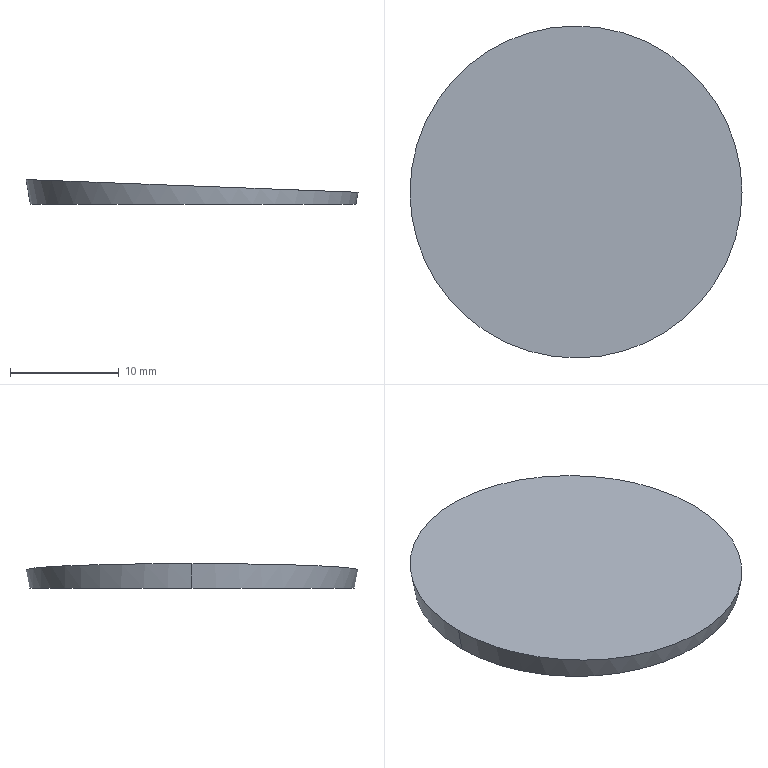Part | Creo | 1 solid | 4 faces | box 30.6 x 30.599 x 2.285 mm | volume 1225 mm3 | plane 2 | cone 2
STEP:
#1=CARTESIAN_POINT('',(15.,35.,35.405));
#2=VERTEX_POINT('',#1);
#3=CARTESIAN_POINT('',(-15.,35.,35.405));
#4=VERTEX_POINT('',#3);
#5=CARTESIAN_POINT('',(0.,35.,35.405));
#6=DIRECTION('',(0.,0.,-1.));
#7=DIRECTION('',(1.,0.,0.));
#8=AXIS2_PLACEMENT_3D('',#5,#6,#7);
#9=CIRCLE('',#8,15.);
#10=EDGE_CURVE('',#2,#4,#9,.T.);
#11=ORIENTED_EDGE('',*,*,#10,.F.);
#12=CARTESIAN_POINT('',(0.,35.,35.405));
#13=DIRECTION('',(0.,0.,-1.));
#14=DIRECTION('',(-1.,0.,0.));
#15=AXIS2_PLACEMENT_3D('',#12,#13,#14);
#16=CIRCLE('',#15,15.);
#17=EDGE_CURVE('',#4,#2,#16,.T.);
#18=ORIENTED_EDGE('',*,*,#17,.F.);
#19=EDGE_LOOP('',(#11,#18));
#20=FACE_OUTER_BOUND('',#19,.F.);
#21=CARTESIAN_POINT('',(0.,35.,35.405));
#22=DIRECTION('',(0.,0.,-1.));
#23=DIRECTION('',(-1.,0.,0.));
#24=AXIS2_PLACEMENT_3D('',#21,#22,#23);
#25=PLANE('',#24);
#26=ADVANCED_FACE('',(#20),#25,.T.);
#27=ORIENTED_EDGE('',*,*,#10,.T.);
#28=CARTESIAN_POINT('',(-15.403,35.,37.69));
#29=VERTEX_POINT('',#28);
#30=CARTESIAN_POINT('',(-15.,35.,35.405));
#31=DIRECTION('',(-0.1736,0.,0.9848));
#32=VECTOR('',#31,2.32);
#33=LINE('',#30,#32);
#34=EDGE_CURVE('',#4,#29,#33,.T.);
#35=ORIENTED_EDGE('',*,*,#34,.T.);
#36=CARTESIAN_POINT('',(15.197,35.,36.522));
#37=VERTEX_POINT('',#36);
#38=CARTESIAN_POINT('',(-15.403,35.,37.69));
#39=CARTESIAN_POINT('',(-15.403,34.098,37.69));
#40=CARTESIAN_POINT('',(-15.243,32.228,37.684));
#41=CARTESIAN_POINT('',(-14.431,29.351,37.653));
#42=CARTESIAN_POINT('',(-13.006,26.578,37.599));
#43=CARTESIAN_POINT('',(-11.,24.103,37.522));
#44=CARTESIAN_POINT('',(-8.525,22.097,37.428));
#45=CARTESIAN_POINT('',(-6.214,20.91,37.34));
#46=CARTESIAN_POINT('',(-4.314,20.266,37.267));
#47=CARTESIAN_POINT('',(-2.884,19.932,37.212));
#48=CARTESIAN_POINT('',(-1.708,19.772,37.168));
#49=CARTESIAN_POINT('',(-0.7827,19.71,37.132));
#50=CARTESIAN_POINT('',(-0.103,19.695,37.106));
#51=CARTESIAN_POINT('',(0.5768,19.71,37.08));
#52=CARTESIAN_POINT('',(1.502,19.772,37.045));
#53=CARTESIAN_POINT('',(2.678,19.932,37.));
#54=CARTESIAN_POINT('',(4.108,20.266,36.946));
#55=CARTESIAN_POINT('',(6.008,20.91,36.873));
#56=CARTESIAN_POINT('',(8.319,22.097,36.785));
#57=CARTESIAN_POINT('',(10.794,24.103,36.69));
#58=CARTESIAN_POINT('',(12.8,26.578,36.614));
#59=CARTESIAN_POINT('',(14.225,29.351,36.559));
#60=CARTESIAN_POINT('',(15.037,32.228,36.528));
#61=CARTESIAN_POINT('',(15.197,34.098,36.522));
#62=CARTESIAN_POINT('',(15.197,35.,36.522));
#63=B_SPLINE_CURVE_WITH_KNOTS('',3,(#38,#39,#40,#41,#42,#43,#44,#45,#46,#47,#48,#49,#50,#51,#52,#53,#54,#55,#56,#57,#58,#59,#60,#61,#62),.UNSPECIFIED.,.F.,.F.,(4,1,1,1,1,1,1,1,1,1,1,1,1,1,1,1,1,1,1,1,1,1,4),(0.,0.0625,0.125,0.1875,0.25,0.3125,0.375,0.4062,0.4375,0.4688,0.4844,0.5,0.5156,0.5312,0.5625,0.5938,0.625,0.6875,0.75,0.8125,0.875,0.9375,1.),.UNSPECIFIED.);
#64=EDGE_CURVE('',#29,#37,#63,.T.);
#65=ORIENTED_EDGE('',*,*,#64,.T.);
#66=CARTESIAN_POINT('',(15.,35.,35.405));
#67=DIRECTION('',(0.1736,0.,0.9848));
#68=VECTOR('',#67,1.134);
#69=LINE('',#66,#68);
#70=EDGE_CURVE('',#2,#37,#69,.T.);
#71=ORIENTED_EDGE('',*,*,#70,.F.);
#72=EDGE_LOOP('',(#27,#35,#65,#71));
#73=FACE_OUTER_BOUND('',#72,.F.);
#74=CARTESIAN_POINT('',(0.,35.,36.548));
#75=DIRECTION('',(0.,0.,1.));
#76=DIRECTION('',(-1.,0.,0.));
#77=AXIS2_PLACEMENT_3D('',#74,#75,#76);
#78=CONICAL_SURFACE('',#77,15.201,10.);
#79=ADVANCED_FACE('',(#73),#78,.T.);
#80=ORIENTED_EDGE('',*,*,#17,.T.);
#81=ORIENTED_EDGE('',*,*,#70,.T.);
#82=CARTESIAN_POINT('',(15.197,35.,36.522));
#83=CARTESIAN_POINT('',(15.197,35.902,36.522));
#84=CARTESIAN_POINT('',(15.037,37.772,36.528));
#85=CARTESIAN_POINT('',(14.225,40.649,36.559));
#86=CARTESIAN_POINT('',(12.8,43.422,36.614));
#87=CARTESIAN_POINT('',(10.794,45.897,36.69));
#88=CARTESIAN_POINT('',(8.319,47.903,36.785));
#89=CARTESIAN_POINT('',(6.008,49.09,36.873));
#90=CARTESIAN_POINT('',(4.108,49.734,36.946));
#91=CARTESIAN_POINT('',(2.678,50.068,37.));
#92=CARTESIAN_POINT('',(1.502,50.228,37.045));
#93=CARTESIAN_POINT('',(0.5768,50.29,37.08));
#94=CARTESIAN_POINT('',(-0.103,50.305,37.106));
#95=CARTESIAN_POINT('',(-0.7827,50.29,37.132));
#96=CARTESIAN_POINT('',(-1.708,50.228,37.168));
#97=CARTESIAN_POINT('',(-2.884,50.068,37.212));
#98=CARTESIAN_POINT('',(-4.314,49.734,37.267));
#99=CARTESIAN_POINT('',(-6.214,49.09,37.34));
#100=CARTESIAN_POINT('',(-8.525,47.903,37.428));
#101=CARTESIAN_POINT('',(-11.,45.897,37.522));
#102=CARTESIAN_POINT('',(-13.006,43.422,37.599));
#103=CARTESIAN_POINT('',(-14.431,40.649,37.653));
#104=CARTESIAN_POINT('',(-15.243,37.772,37.684));
#105=CARTESIAN_POINT('',(-15.403,35.902,37.69));
#106=CARTESIAN_POINT('',(-15.403,35.,37.69));
#107=B_SPLINE_CURVE_WITH_KNOTS('',3,(#82,#83,#84,#85,#86,#87,#88,#89,#90,#91,#92,#93,#94,#95,#96,#97,#98,#99,#100,#101,#102,#103,#104,#105,#106),.UNSPECIFIED.,.F.,.F.,(4,1,1,1,1,1,1,1,1,1,1,1,1,1,1,1,1,1,1,1,1,1,4),(0.,0.0625,0.125,0.1875,0.25,0.3125,0.375,0.4062,0.4375,0.4688,0.4844,0.5,0.5156,0.5312,0.5625,0.5938,0.625,0.6875,0.75,0.8125,0.875,0.9375,1.),.UNSPECIFIED.);
#108=EDGE_CURVE('',#37,#29,#107,.T.);
#109=ORIENTED_EDGE('',*,*,#108,.T.);
#110=ORIENTED_EDGE('',*,*,#34,.F.);
#111=EDGE_LOOP('',(#80,#81,#109,#110));
#112=FACE_OUTER_BOUND('',#111,.F.);
#113=CARTESIAN_POINT('',(0.,35.,36.548));
#114=DIRECTION('',(0.,0.,1.));
#115=DIRECTION('',(-1.,0.,0.));
#116=AXIS2_PLACEMENT_3D('',#113,#114,#115);
#117=CONICAL_SURFACE('',#116,15.201,10.);
#118=ADVANCED_FACE('',(#112),#117,.T.);
#119=ORIENTED_EDGE('',*,*,#64,.F.);
#120=ORIENTED_EDGE('',*,*,#108,.F.);
#121=EDGE_LOOP('',(#119,#120));
#122=FACE_OUTER_BOUND('',#121,.F.);
#123=CARTESIAN_POINT('',(-120.707,-167.242,41.71));
#124=DIRECTION('',(-0.03814,0.,-0.9993));
#125=DIRECTION('',(-0.9993,0.,0.03814));
#126=AXIS2_PLACEMENT_3D('',#123,#124,#125);
#127=PLANE('',#126);
#128=ADVANCED_FACE('',(#122),#127,.F.);
#129=CLOSED_SHELL('',(#26,#79,#118,#128));
#130=MANIFOLD_SOLID_BREP('',#129);
#131=(LENGTH_UNIT()NAMED_UNIT(*)SI_UNIT(.MILLI.,.METRE.));
#132=UNCERTAINTY_MEASURE_WITH_UNIT(LENGTH_MEASURE(0.004362),#131,'','');
#133=(NAMED_UNIT(*)PLANE_ANGLE_UNIT()SI_UNIT($,.RADIAN.));
#134=PLANE_ANGLE_MEASURE_WITH_UNIT(PLANE_ANGLE_MEASURE(0.01745),#133);
#135=(CONVERSION_BASED_UNIT('DEGREE',#134)NAMED_UNIT(*)PLANE_ANGLE_UNIT());
#136=(NAMED_UNIT(*)SI_UNIT($,.STERADIAN.)SOLID_ANGLE_UNIT());
#137=(GEOMETRIC_REPRESENTATION_CONTEXT(3)GLOBAL_UNCERTAINTY_ASSIGNED_CONTEXT((#132))GLOBAL_UNIT_ASSIGNED_CONTEXT((#131,#135,#136))REPRESENTATION_CONTEXT('',''));
#138=ADVANCED_BREP_SHAPE_REPRESENTATION('',(#130),#137);